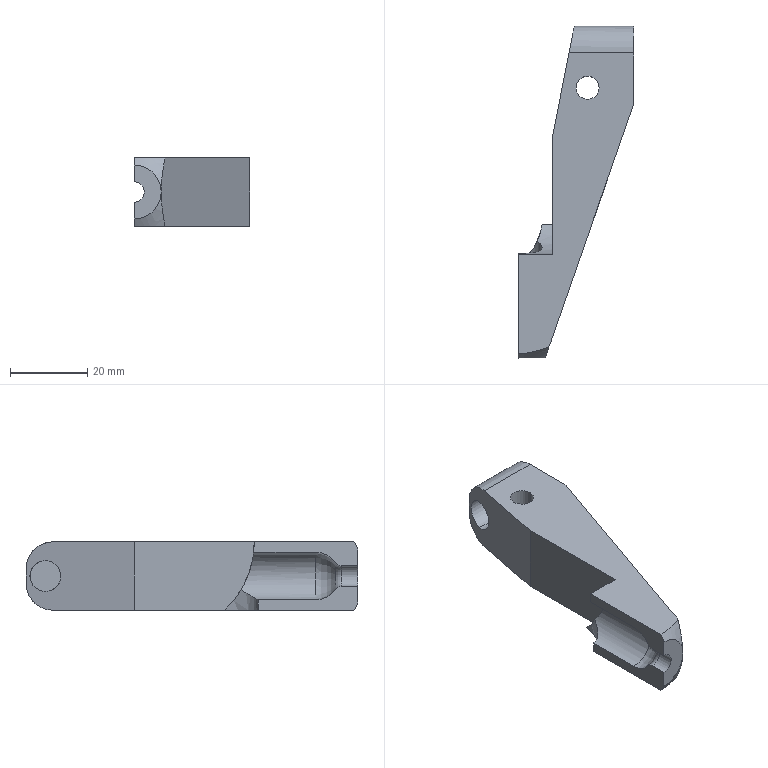Part | SolidWorks | features ICE 6, Extrusion 1, Fillet 1, RevCut 1 | 1 solid | 25 faces | box 30 x 86 x 17.7 mm | volume 18954 mm3 | plane 11 | cylinder 8 | spline 2 | torus 2 | cone 2 | commonest cylinder face diameters 6 x2 8 x2 14 x2 5.3 x1 12.388 x1
STEP:
#1=CARTESIAN_POINT('',(54.,-5.,4.85));
#2=VERTEX_POINT('',#1);
#3=CARTESIAN_POINT('',(54.,-5.,12.85));
#4=VERTEX_POINT('',#3);
#5=CARTESIAN_POINT('',(54.,-5.,8.85));
#6=DIRECTION('',(-1.,0.,0.));
#7=DIRECTION('',(0.,0.,1.));
#8=AXIS2_PLACEMENT_3D('',#5,#6,#7);
#9=CIRCLE('',#8,4.);
#10=EDGE_CURVE('',#2,#4,#9,.T.);
#11=ORIENTED_EDGE('',*,*,#10,.F.);
#12=CARTESIAN_POINT('',(43.6,-5.,4.85));
#13=VERTEX_POINT('',#12);
#14=CARTESIAN_POINT('',(54.,-5.,4.85));
#15=DIRECTION('',(-1.,0.,0.));
#16=VECTOR('',#15,1000.);
#17=LINE('',#14,#16);
#18=EDGE_CURVE('',#2,#13,#17,.T.);
#19=ORIENTED_EDGE('',*,*,#18,.T.);
#20=CARTESIAN_POINT('',(43.6,-5.,12.85));
#21=VERTEX_POINT('',#20);
#22=CARTESIAN_POINT('',(43.6,-5.,12.85));
#23=CARTESIAN_POINT('',(42.,-13.,12.85));
#24=CARTESIAN_POINT('',(42.,-13.,4.85));
#25=CARTESIAN_POINT('',(43.6,-5.,4.85));
#26=(BOUNDED_CURVE()B_SPLINE_CURVE(3,(#22,#23,#24,#25),.UNSPECIFIED.,.F.,.F.)B_SPLINE_CURVE_WITH_KNOTS((4,4),(4.712,7.854),.UNSPECIFIED.)CURVE()GEOMETRIC_REPRESENTATION_ITEM()RATIONAL_B_SPLINE_CURVE((1.,0.3333,0.3333,1.))REPRESENTATION_ITEM(''));
#27=EDGE_CURVE('',#21,#13,#26,.T.);
#28=ORIENTED_EDGE('',*,*,#27,.F.);
#29=CARTESIAN_POINT('',(54.,-5.,12.85));
#30=DIRECTION('',(-1.,0.,0.));
#31=VECTOR('',#30,1000.);
#32=LINE('',#29,#31);
#33=EDGE_CURVE('',#4,#21,#32,.T.);
#34=ORIENTED_EDGE('',*,*,#33,.F.);
#35=EDGE_LOOP('',(#11,#19,#28,#34));
#36=FACE_OUTER_BOUND('',#35,.T.);
#37=CARTESIAN_POINT('',(54.,-5.,8.85));
#38=DIRECTION('',(-1.,0.,0.));
#39=DIRECTION('',(0.,0.,1.));
#40=AXIS2_PLACEMENT_3D('',#37,#38,#39);
#41=CYLINDRICAL_SURFACE('',#40,4.);
#42=ADVANCED_FACE('',(#36),#41,.F.);
#43=CARTESIAN_POINT('',(45.,-16.,17.7));
#44=VERTEX_POINT('',#43);
#45=CARTESIAN_POINT('',(51.,-16.,17.7));
#46=VERTEX_POINT('',#45);
#47=CARTESIAN_POINT('',(48.,-16.,17.7));
#48=DIRECTION('',(0.,0.,1.));
#49=DIRECTION('',(1.,0.,0.));
#50=AXIS2_PLACEMENT_3D('',#47,#48,#49);
#51=CIRCLE('',#50,3.);
#52=EDGE_CURVE('',#44,#46,#51,.T.);
#53=ORIENTED_EDGE('',*,*,#52,.T.);
#54=CARTESIAN_POINT('',(51.,-16.,0.));
#55=VERTEX_POINT('',#54);
#56=CARTESIAN_POINT('',(51.,-16.,17.7));
#57=DIRECTION('',(0.,0.,-1.));
#58=VECTOR('',#57,1000.);
#59=LINE('',#56,#58);
#60=EDGE_CURVE('',#46,#55,#59,.T.);
#61=ORIENTED_EDGE('',*,*,#60,.T.);
#62=CARTESIAN_POINT('',(45.,-16.,0.));
#63=VERTEX_POINT('',#62);
#64=CARTESIAN_POINT('',(48.,-16.,0.));
#65=DIRECTION('',(0.,0.,1.));
#66=DIRECTION('',(1.,0.,0.));
#67=AXIS2_PLACEMENT_3D('',#64,#65,#66);
#68=CIRCLE('',#67,3.);
#69=EDGE_CURVE('',#63,#55,#68,.T.);
#70=ORIENTED_EDGE('',*,*,#69,.F.);
#71=CARTESIAN_POINT('',(45.,-16.,17.7));
#72=DIRECTION('',(0.,0.,-1.));
#73=VECTOR('',#72,1000.);
#74=LINE('',#71,#73);
#75=EDGE_CURVE('',#44,#63,#74,.T.);
#76=ORIENTED_EDGE('',*,*,#75,.F.);
#77=EDGE_LOOP('',(#53,#61,#70,#76));
#78=FACE_OUTER_BOUND('',#77,.T.);
#79=CARTESIAN_POINT('',(48.,-16.,17.7));
#80=DIRECTION('',(0.,0.,-1.));
#81=DIRECTION('',(-1.,0.,0.));
#82=AXIS2_PLACEMENT_3D('',#79,#80,#81);
#83=CYLINDRICAL_SURFACE('',#82,3.);
#84=ADVANCED_FACE('',(#78),#83,.F.);
#85=CARTESIAN_POINT('',(30.,-84.932,17.7));
#86=VERTEX_POINT('',#85);
#87=CARTESIAN_POINT('',(30.,-59.152,17.7));
#88=VERTEX_POINT('',#87);
#89=CARTESIAN_POINT('',(30.,-86.,17.7));
#90=DIRECTION('',(0.,1.,0.));
#91=VECTOR('',#90,1000.);
#92=LINE('',#89,#91);
#93=EDGE_CURVE('',#86,#88,#92,.T.);
#94=ORIENTED_EDGE('',*,*,#93,.F.);
#95=CARTESIAN_POINT('',(37.993,-83.156,17.7));
#96=VERTEX_POINT('',#95);
#97=CARTESIAN_POINT('',(30.,-84.932,17.7));
#98=CARTESIAN_POINT('',(30.683,-84.932,17.7));
#99=CARTESIAN_POINT('',(31.369,-84.886,17.7));
#100=CARTESIAN_POINT('',(32.745,-84.706,17.7));
#101=CARTESIAN_POINT('',(33.421,-84.575,17.7));
#102=CARTESIAN_POINT('',(35.419,-84.091,17.7));
#103=CARTESIAN_POINT('',(36.715,-83.651,17.7));
#104=CARTESIAN_POINT('',(37.993,-83.156,17.7));
#105=B_SPLINE_CURVE_WITH_KNOTS('',3,(#97,#98,#99,#100,#101,#102,#103,#104),.UNSPECIFIED.,.F.,.F.,(4,2,2,4),(0.1214,0.1235,0.1255,0.1297),.UNSPECIFIED.);
#106=EDGE_CURVE('',#86,#96,#105,.T.);
#107=ORIENTED_EDGE('',*,*,#106,.T.);
#108=CARTESIAN_POINT('',(38.331,-82.189,17.7));
#109=VERTEX_POINT('',#108);
#110=CARTESIAN_POINT('',(37.993,-83.156,17.7));
#111=CARTESIAN_POINT('',(38.103,-82.841,17.7));
#112=CARTESIAN_POINT('',(38.216,-82.517,17.7));
#113=CARTESIAN_POINT('',(38.331,-82.189,17.7));
#114=B_SPLINE_CURVE_WITH_KNOTS('',3,(#110,#111,#112,#113),.UNSPECIFIED.,.F.,.F.,(4,4),(0.3587,0.5),.UNSPECIFIED.);
#115=EDGE_CURVE('',#96,#109,#114,.T.);
#116=ORIENTED_EDGE('',*,*,#115,.T.);
#117=CARTESIAN_POINT('',(38.951,-80.412,17.7));
#118=VERTEX_POINT('',#117);
#119=CARTESIAN_POINT('',(38.331,-82.189,17.7));
#120=CARTESIAN_POINT('',(38.533,-81.609,17.7));
#121=CARTESIAN_POINT('',(38.741,-81.014,17.7));
#122=CARTESIAN_POINT('',(38.951,-80.412,17.7));
#123=B_SPLINE_CURVE_WITH_KNOTS('',3,(#119,#120,#121,#122),.UNSPECIFIED.,.F.,.F.,(4,4),(0.,0.25),.UNSPECIFIED.);
#124=EDGE_CURVE('',#109,#118,#123,.T.);
#125=ORIENTED_EDGE('',*,*,#124,.T.);
#126=CARTESIAN_POINT('',(60.,-20.136,17.7));
#127=VERTEX_POINT('',#126);
#128=CARTESIAN_POINT('',(60.,-20.136,17.7));
#129=DIRECTION('',(0.3297,0.9441,0.));
#130=VECTOR('',#129,1000.);
#131=LINE('',#128,#130);
#132=EDGE_CURVE('',#118,#127,#131,.T.);
#133=ORIENTED_EDGE('',*,*,#132,.T.);
#134=CARTESIAN_POINT('',(60.,-7.,17.7));
#135=VERTEX_POINT('',#134);
#136=CARTESIAN_POINT('',(60.,-20.136,17.7));
#137=DIRECTION('',(0.,1.,0.));
#138=VECTOR('',#137,1000.);
#139=LINE('',#136,#138);
#140=EDGE_CURVE('',#127,#135,#139,.T.);
#141=ORIENTED_EDGE('',*,*,#140,.T.);
#142=CARTESIAN_POINT('',(43.2,-7.,17.7));
#143=VERTEX_POINT('',#142);
#144=CARTESIAN_POINT('',(44.6,-7.,17.7));
#145=DIRECTION('',(-1.,0.,0.));
#146=VECTOR('',#145,1000.);
#147=LINE('',#144,#146);
#148=EDGE_CURVE('',#135,#143,#147,.T.);
#149=ORIENTED_EDGE('',*,*,#148,.T.);
#150=CARTESIAN_POINT('',(39.,-28.,17.7));
#151=VERTEX_POINT('',#150);
#152=CARTESIAN_POINT('',(44.6,0.,17.7));
#153=DIRECTION('',(-0.1961,-0.9806,0.));
#154=VECTOR('',#153,1000.);
#155=LINE('',#152,#154);
#156=EDGE_CURVE('',#143,#151,#155,.T.);
#157=ORIENTED_EDGE('',*,*,#156,.T.);
#158=CARTESIAN_POINT('',(39.,-59.152,17.7));
#159=VERTEX_POINT('',#158);
#160=CARTESIAN_POINT('',(39.,-28.,17.7));
#161=DIRECTION('',(0.,-1.,0.));
#162=VECTOR('',#161,1000.);
#163=LINE('',#160,#162);
#164=EDGE_CURVE('',#151,#159,#163,.T.);
#165=ORIENTED_EDGE('',*,*,#164,.T.);
#166=CARTESIAN_POINT('',(58.282,-59.152,17.7));
#167=DIRECTION('',(-1.,0.,0.));
#168=VECTOR('',#167,1000.);
#169=LINE('',#166,#168);
#170=EDGE_CURVE('',#159,#88,#169,.T.);
#171=ORIENTED_EDGE('',*,*,#170,.T.);
#172=EDGE_LOOP('',(#94,#107,#116,#125,#133,#141,#149,#157,#165,#171));
#173=FACE_OUTER_BOUND('',#172,.T.);
#174=ORIENTED_EDGE('',*,*,#52,.F.);
#175=CARTESIAN_POINT('',(48.,-16.,17.7));
#176=DIRECTION('',(0.,0.,1.));
#177=DIRECTION('',(1.,0.,0.));
#178=AXIS2_PLACEMENT_3D('',#175,#176,#177);
#179=CIRCLE('',#178,3.);
#180=EDGE_CURVE('',#46,#44,#179,.T.);
#181=ORIENTED_EDGE('',*,*,#180,.F.);
#182=EDGE_LOOP('',(#174,#181));
#183=FACE_BOUND('',#182,.T.);
#184=CARTESIAN_POINT('',(25.162,-51.504,17.7));
#185=DIRECTION('',(0.,0.,1.));
#186=DIRECTION('',(1.,0.,0.));
#187=AXIS2_PLACEMENT_3D('',#184,#185,#186);
#188=PLANE('',#187);
#189=ADVANCED_FACE('',(#173,#183),#188,.T.);
#190=ORIENTED_EDGE('',*,*,#69,.T.);
#191=CARTESIAN_POINT('',(48.,-16.,0.));
#192=DIRECTION('',(0.,0.,1.));
#193=DIRECTION('',(1.,0.,0.));
#194=AXIS2_PLACEMENT_3D('',#191,#192,#193);
#195=CIRCLE('',#194,3.);
#196=EDGE_CURVE('',#55,#63,#195,.T.);
#197=ORIENTED_EDGE('',*,*,#196,.T.);
#198=EDGE_LOOP('',(#190,#197));
#199=FACE_BOUND('',#198,.T.);
#200=CARTESIAN_POINT('',(30.,-84.932,0.));
#201=VERTEX_POINT('',#200);
#202=CARTESIAN_POINT('',(37.993,-83.156,-0.000000005));
#203=VERTEX_POINT('',#202);
#204=CARTESIAN_POINT('',(30.,-84.932,0.));
#205=CARTESIAN_POINT('',(30.683,-84.932,0.));
#206=CARTESIAN_POINT('',(31.369,-84.886,0.));
#207=CARTESIAN_POINT('',(32.745,-84.706,0.));
#208=CARTESIAN_POINT('',(33.421,-84.575,0.));
#209=CARTESIAN_POINT('',(35.419,-84.091,0.));
#210=CARTESIAN_POINT('',(36.715,-83.651,0.));
#211=CARTESIAN_POINT('',(37.993,-83.156,-0.000000005));
#212=B_SPLINE_CURVE_WITH_KNOTS('',3,(#204,#205,#206,#207,#208,#209,#210,#211),.UNSPECIFIED.,.F.,.F.,(4,2,2,4),(0.1214,0.1235,0.1255,0.1297),.UNSPECIFIED.);
#213=EDGE_CURVE('',#201,#203,#212,.T.);
#214=ORIENTED_EDGE('',*,*,#213,.F.);
#215=CARTESIAN_POINT('',(30.,-60.226,0.));
#216=VERTEX_POINT('',#215);
#217=CARTESIAN_POINT('',(30.,-51.504,0.));
#218=DIRECTION('',(0.,1.,0.));
#219=VECTOR('',#218,1000.);
#220=LINE('',#217,#219);
#221=EDGE_CURVE('',#201,#216,#220,.T.);
#222=ORIENTED_EDGE('',*,*,#221,.T.);
#223=CARTESIAN_POINT('',(36.216,-51.504,0.));
#224=VERTEX_POINT('',#223);
#225=CARTESIAN_POINT('',(36.216,-51.504,0.));
#226=CARTESIAN_POINT('',(35.359,-56.878,0.));
#227=CARTESIAN_POINT('',(32.973,-60.226,0.));
#228=CARTESIAN_POINT('',(30.,-60.226,0.));
#229=(BOUNDED_CURVE()B_SPLINE_CURVE(3,(#225,#226,#227,#228),.UNSPECIFIED.,.F.,.F.)B_SPLINE_CURVE_WITH_KNOTS((4,4),(1.863,3.142),.UNSPECIFIED.)CURVE()GEOMETRIC_REPRESENTATION_ITEM()RATIONAL_B_SPLINE_CURVE((1.,0.8684,0.8684,1.))REPRESENTATION_ITEM(''));
#230=EDGE_CURVE('',#224,#216,#229,.T.);
#231=ORIENTED_EDGE('',*,*,#230,.F.);
#232=CARTESIAN_POINT('',(39.,-51.504,0.));
#233=VERTEX_POINT('',#232);
#234=CARTESIAN_POINT('',(39.,-51.504,0.));
#235=DIRECTION('',(-1.,0.,0.));
#236=VECTOR('',#235,1000.);
#237=LINE('',#234,#236);
#238=EDGE_CURVE('',#233,#224,#237,.T.);
#239=ORIENTED_EDGE('',*,*,#238,.F.);
#240=CARTESIAN_POINT('',(39.,-28.,0.));
#241=VERTEX_POINT('',#240);
#242=CARTESIAN_POINT('',(39.,-28.,0.));
#243=DIRECTION('',(0.,-1.,0.));
#244=VECTOR('',#243,1000.);
#245=LINE('',#242,#244);
#246=EDGE_CURVE('',#241,#233,#245,.T.);
#247=ORIENTED_EDGE('',*,*,#246,.F.);
#248=CARTESIAN_POINT('',(43.2,-7.,0.));
#249=VERTEX_POINT('',#248);
#250=CARTESIAN_POINT('',(44.6,0.,0.));
#251=DIRECTION('',(-0.1961,-0.9806,0.));
#252=VECTOR('',#251,1000.);
#253=LINE('',#250,#252);
#254=EDGE_CURVE('',#249,#241,#253,.T.);
#255=ORIENTED_EDGE('',*,*,#254,.F.);
#256=CARTESIAN_POINT('',(60.,-7.,0.));
#257=VERTEX_POINT('',#256);
#258=CARTESIAN_POINT('',(25.162,-7.,0.));
#259=DIRECTION('',(1.,0.,0.));
#260=VECTOR('',#259,1000.);
#261=LINE('',#258,#260);
#262=EDGE_CURVE('',#249,#257,#261,.T.);
#263=ORIENTED_EDGE('',*,*,#262,.T.);
#264=CARTESIAN_POINT('',(60.,-20.136,0.));
#265=VERTEX_POINT('',#264);
#266=CARTESIAN_POINT('',(60.,-20.136,0.));
#267=DIRECTION('',(0.,1.,0.));
#268=VECTOR('',#267,1000.);
#269=LINE('',#266,#268);
#270=EDGE_CURVE('',#265,#257,#269,.T.);
#271=ORIENTED_EDGE('',*,*,#270,.F.);
#272=CARTESIAN_POINT('',(38.951,-80.412,0.));
#273=VERTEX_POINT('',#272);
#274=CARTESIAN_POINT('',(60.,-20.136,0.));
#275=DIRECTION('',(0.3297,0.9441,0.));
#276=VECTOR('',#275,1000.);
#277=LINE('',#274,#276);
#278=EDGE_CURVE('',#273,#265,#277,.T.);
#279=ORIENTED_EDGE('',*,*,#278,.F.);
#280=CARTESIAN_POINT('',(38.331,-82.189,0.));
#281=VERTEX_POINT('',#280);
#282=CARTESIAN_POINT('',(38.331,-82.189,0.));
#283=CARTESIAN_POINT('',(38.533,-81.609,0.));
#284=CARTESIAN_POINT('',(38.741,-81.014,0.));
#285=CARTESIAN_POINT('',(38.951,-80.412,0.));
#286=B_SPLINE_CURVE_WITH_KNOTS('',3,(#282,#283,#284,#285),.UNSPECIFIED.,.F.,.F.,(4,4),(0.,0.25),.UNSPECIFIED.);
#287=EDGE_CURVE('',#281,#273,#286,.T.);
#288=ORIENTED_EDGE('',*,*,#287,.F.);
#289=CARTESIAN_POINT('',(37.993,-83.156,-0.000000005));
#290=CARTESIAN_POINT('',(38.103,-82.841,0.));
#291=CARTESIAN_POINT('',(38.216,-82.517,0.));
#292=CARTESIAN_POINT('',(38.331,-82.189,0.));
#293=B_SPLINE_CURVE_WITH_KNOTS('',3,(#289,#290,#291,#292),.UNSPECIFIED.,.F.,.F.,(4,4),(0.3587,0.5),.UNSPECIFIED.);
#294=EDGE_CURVE('',#203,#281,#293,.T.);
#295=ORIENTED_EDGE('',*,*,#294,.F.);
#296=EDGE_LOOP('',(#214,#222,#231,#239,#247,#255,#263,#271,#279,#288,#295));
#297=FACE_OUTER_BOUND('',#296,.T.);
#298=CARTESIAN_POINT('',(25.162,-51.504,0.));
#299=DIRECTION('',(0.,0.,1.));
#300=DIRECTION('',(1.,0.,0.));
#301=AXIS2_PLACEMENT_3D('',#298,#299,#300);
#302=PLANE('',#301);
#303=ADVANCED_FACE('',(#199,#297),#302,.F.);
#304=CARTESIAN_POINT('',(37.,-86.,8.85));
#305=VERTEX_POINT('',#304);
#306=CARTESIAN_POINT('',(30.,-86.,15.85));
#307=VERTEX_POINT('',#306);
#308=CARTESIAN_POINT('',(30.,-86.,8.85));
#309=DIRECTION('',(0.,-1.,0.));
#310=DIRECTION('',(0.,0.,-1.));
#311=AXIS2_PLACEMENT_3D('',#308,#309,#310);
#312=CIRCLE('',#311,7.);
#313=EDGE_CURVE('',#305,#307,#312,.T.);
#314=ORIENTED_EDGE('',*,*,#313,.T.);
#315=CARTESIAN_POINT('',(30.,-86.,11.5));
#316=VERTEX_POINT('',#315);
#317=CARTESIAN_POINT('',(30.,-86.,-26.3));
#318=DIRECTION('',(0.,0.,1.));
#319=VECTOR('',#318,1000.);
#320=LINE('',#317,#319);
#321=EDGE_CURVE('',#316,#307,#320,.T.);
#322=ORIENTED_EDGE('',*,*,#321,.F.);
#323=CARTESIAN_POINT('',(30.,-86.,6.2));
#324=VERTEX_POINT('',#323);
#325=CARTESIAN_POINT('',(30.,-86.,8.85));
#326=DIRECTION('',(0.,-1.,0.));
#327=DIRECTION('',(0.,0.,-1.));
#328=AXIS2_PLACEMENT_3D('',#325,#326,#327);
#329=CIRCLE('',#328,2.65);
#330=EDGE_CURVE('',#324,#316,#329,.T.);
#331=ORIENTED_EDGE('',*,*,#330,.F.);
#332=CARTESIAN_POINT('',(30.,-86.,1.85));
#333=VERTEX_POINT('',#332);
#334=CARTESIAN_POINT('',(30.,-86.,-26.3));
#335=DIRECTION('',(0.,0.,1.));
#336=VECTOR('',#335,1000.);
#337=LINE('',#334,#336);
#338=EDGE_CURVE('',#333,#324,#337,.T.);
#339=ORIENTED_EDGE('',*,*,#338,.F.);
#340=CARTESIAN_POINT('',(30.,-86.,8.85));
#341=DIRECTION('',(0.,-1.,0.));
#342=DIRECTION('',(0.,0.,-1.));
#343=AXIS2_PLACEMENT_3D('',#340,#341,#342);
#344=CIRCLE('',#343,7.);
#345=EDGE_CURVE('',#333,#305,#344,.T.);
#346=ORIENTED_EDGE('',*,*,#345,.T.);
#347=EDGE_LOOP('',(#314,#322,#331,#339,#346));
#348=FACE_OUTER_BOUND('',#347,.T.);
#349=CARTESIAN_POINT('',(37.,-86.,17.7));
#350=DIRECTION('',(0.,1.,0.));
#351=DIRECTION('',(0.,0.,1.));
#352=AXIS2_PLACEMENT_3D('',#349,#350,#351);
#353=PLANE('',#352);
#354=ADVANCED_FACE('',(#348),#353,.F.);
#355=CARTESIAN_POINT('',(37.993,-83.156,-0.000000005));
#356=CARTESIAN_POINT('',(37.872,-83.502,0.6974));
#357=CARTESIAN_POINT('',(37.755,-83.838,1.399));
#358=CARTESIAN_POINT('',(37.532,-84.477,2.819));
#359=CARTESIAN_POINT('',(37.426,-84.78,3.537));
#360=CARTESIAN_POINT('',(37.237,-85.321,5.003));
#361=CARTESIAN_POINT('',(37.154,-85.56,5.755));
#362=CARTESIAN_POINT('',(37.035,-85.9,7.28));
#363=CARTESIAN_POINT('',(37.,-86.,8.056));
#364=CARTESIAN_POINT('',(37.,-86.,8.85));
#365=B_SPLINE_CURVE_WITH_KNOTS('',3,(#355,#356,#357,#358,#359,#360,#361,#362,#363,#364),.UNSPECIFIED.,.F.,.F.,(4,2,2,2,4),(0.000000225,0.002359,0.004717,0.007076,0.009434),.UNSPECIFIED.);
#366=EDGE_CURVE('',#203,#305,#365,.T.);
#367=ORIENTED_EDGE('',*,*,#366,.F.);
#368=ORIENTED_EDGE('',*,*,#294,.T.);
#369=ORIENTED_EDGE('',*,*,#287,.T.);
#370=ORIENTED_EDGE('',*,*,#278,.T.);
#371=CARTESIAN_POINT('',(60.,-20.136,17.7));
#372=DIRECTION('',(0.,0.,-1.));
#373=VECTOR('',#372,1000.);
#374=LINE('',#371,#373);
#375=EDGE_CURVE('',#127,#265,#374,.T.);
#376=ORIENTED_EDGE('',*,*,#375,.F.);
#377=ORIENTED_EDGE('',*,*,#132,.F.);
#378=ORIENTED_EDGE('',*,*,#124,.F.);
#379=ORIENTED_EDGE('',*,*,#115,.F.);
#380=CARTESIAN_POINT('',(37.,-86.,8.85));
#381=CARTESIAN_POINT('',(37.,-86.,9.644));
#382=CARTESIAN_POINT('',(37.035,-85.9,10.421));
#383=CARTESIAN_POINT('',(37.154,-85.56,11.945));
#384=CARTESIAN_POINT('',(37.237,-85.321,12.697));
#385=CARTESIAN_POINT('',(37.426,-84.78,14.163));
#386=CARTESIAN_POINT('',(37.532,-84.477,14.881));
#387=CARTESIAN_POINT('',(37.755,-83.838,16.301));
#388=CARTESIAN_POINT('',(37.872,-83.502,17.003));
#389=CARTESIAN_POINT('',(37.993,-83.156,17.7));
#390=B_SPLINE_CURVE_WITH_KNOTS('',3,(#380,#381,#382,#383,#384,#385,#386,#387,#388,#389),.UNSPECIFIED.,.F.,.F.,(4,2,2,2,4),(0.009434,0.01179,0.01415,0.01651,0.01886),.UNSPECIFIED.);
#391=EDGE_CURVE('',#305,#96,#390,.T.);
#392=ORIENTED_EDGE('',*,*,#391,.F.);
#393=EDGE_LOOP('',(#367,#368,#369,#370,#376,#377,#378,#379,#392));
#394=FACE_OUTER_BOUND('',#393,.T.);
#395=CARTESIAN_POINT('',(60.,-20.136,17.7));
#396=DIRECTION('',(-0.9441,0.3297,0.));
#397=DIRECTION('',(-0.3297,-0.9441,0.));
#398=AXIS2_PLACEMENT_3D('',#395,#396,#397);
#399=PLANE('',#398);
#400=ADVANCED_FACE('',(#394),#399,.F.);
#401=CARTESIAN_POINT('',(30.,-75.,2.656));
#402=VERTEX_POINT('',#401);
#403=CARTESIAN_POINT('',(30.,-75.,15.044));
#404=VERTEX_POINT('',#403);
#405=CARTESIAN_POINT('',(30.,-75.,8.85));
#406=DIRECTION('',(0.,-1.,0.));
#407=DIRECTION('',(0.,0.,-1.));
#408=AXIS2_PLACEMENT_3D('',#405,#406,#407);
#409=CIRCLE('',#408,6.194);
#410=EDGE_CURVE('',#402,#404,#409,.T.);
#411=ORIENTED_EDGE('',*,*,#410,.T.);
#412=CARTESIAN_POINT('',(30.,-58.989,15.044));
#413=VERTEX_POINT('',#412);
#414=CARTESIAN_POINT('',(30.,-86.,15.044));
#415=DIRECTION('',(0.,1.,0.));
#416=VECTOR('',#415,1000.);
#417=LINE('',#414,#416);
#418=EDGE_CURVE('',#404,#413,#417,.T.);
#419=ORIENTED_EDGE('',*,*,#418,.T.);
#420=CARTESIAN_POINT('',(35.037,-55.701,5.246));
#421=VERTEX_POINT('',#420);
#422=CARTESIAN_POINT('',(30.,-58.989,15.044));
#423=CARTESIAN_POINT('',(30.294,-58.989,15.044));
#424=CARTESIAN_POINT('',(30.592,-58.987,15.023));
#425=CARTESIAN_POINT('',(31.177,-58.977,14.938));
#426=CARTESIAN_POINT('',(31.464,-58.97,14.876));
#427=CARTESIAN_POINT('',(32.027,-58.95,14.711));
#428=CARTESIAN_POINT('',(32.302,-58.937,14.608));
#429=CARTESIAN_POINT('',(32.842,-58.905,14.362));
#430=CARTESIAN_POINT('',(33.101,-58.885,14.22));
#431=CARTESIAN_POINT('',(33.593,-58.838,13.904));
#432=CARTESIAN_POINT('',(33.827,-58.81,13.729));
#433=CARTESIAN_POINT('',(34.271,-58.744,13.346));
#434=CARTESIAN_POINT('',(34.481,-58.706,13.136));
#435=CARTESIAN_POINT('',(34.864,-58.619,12.697));
#436=CARTESIAN_POINT('',(35.038,-58.571,12.466));
#437=CARTESIAN_POINT('',(35.352,-58.46,11.981));
#438=CARTESIAN_POINT('',(35.493,-58.398,11.726));
#439=CARTESIAN_POINT('',(35.858,-58.193,10.943));
#440=CARTESIAN_POINT('',(36.023,-58.033,10.403));
#441=CARTESIAN_POINT('',(36.204,-57.656,9.292));
#442=CARTESIAN_POINT('',(36.216,-57.441,8.73));
#443=CARTESIAN_POINT('',(36.102,-56.982,7.655));
#444=CARTESIAN_POINT('',(35.976,-56.737,7.137));
#445=CARTESIAN_POINT('',(35.594,-56.221,6.137));
#446=CARTESIAN_POINT('',(35.345,-55.96,5.675));
#447=CARTESIAN_POINT('',(35.037,-55.701,5.246));
#448=B_SPLINE_CURVE_WITH_KNOTS('',3,(#422,#423,#424,#425,#426,#427,#428,#429,#430,#431,#432,#433,#434,#435,#436,#437,#438,#439,#440,#441,#442,#443,#444,#445,#446,#447),.UNSPECIFIED.,.F.,.F.,(4,2,2,2,2,2,2,2,2,2,2,2,4),(0.009865,0.01074,0.01162,0.0125,0.01338,0.01426,0.01514,0.01602,0.0169,0.01866,0.02042,0.02218,0.02394),.UNSPECIFIED.);
#449=EDGE_CURVE('',#413,#421,#448,.T.);
#450=ORIENTED_EDGE('',*,*,#449,.T.);
#451=CARTESIAN_POINT('',(30.,-60.226,2.656));
#452=VERTEX_POINT('',#451);
#453=CARTESIAN_POINT('',(30.,-60.226,2.656));
#454=CARTESIAN_POINT('',(30.16,-60.226,2.656));
#455=CARTESIAN_POINT('',(30.319,-60.215,2.662));
#456=CARTESIAN_POINT('',(30.636,-60.171,2.687));
#457=CARTESIAN_POINT('',(30.794,-60.138,2.705));
#458=CARTESIAN_POINT('',(31.101,-60.052,2.752));
#459=CARTESIAN_POINT('',(31.249,-60.,2.781));
#460=CARTESIAN_POINT('',(31.54,-59.88,2.849));
#461=CARTESIAN_POINT('',(31.682,-59.811,2.887));
#462=CARTESIAN_POINT('',(32.09,-59.586,3.012));
#463=CARTESIAN_POINT('',(32.34,-59.413,3.109));
#464=CARTESIAN_POINT('',(32.807,-59.032,3.322));
#465=CARTESIAN_POINT('',(33.025,-58.823,3.44));
#466=CARTESIAN_POINT('',(33.427,-58.388,3.685));
#467=CARTESIAN_POINT('',(33.612,-58.161,3.814));
#468=CARTESIAN_POINT('',(33.958,-57.693,4.081));
#469=CARTESIAN_POINT('',(34.119,-57.45,4.22));
#470=CARTESIAN_POINT('',(34.566,-56.714,4.645));
#471=CARTESIAN_POINT('',(34.818,-56.21,4.939));
#472=CARTESIAN_POINT('',(35.037,-55.701,5.246));
#473=B_SPLINE_CURVE_WITH_KNOTS('',3,(#453,#454,#455,#456,#457,#458,#459,#460,#461,#462,#463,#464,#465,#466,#467,#468,#469,#470,#471,#472),.UNSPECIFIED.,.F.,.F.,(4,2,2,2,2,2,2,2,2,4),(0.005376,0.005854,0.006331,0.006809,0.007286,0.008241,0.009196,0.01015,0.01111,0.01302),.UNSPECIFIED.);
#474=EDGE_CURVE('',#452,#421,#473,.T.);
#475=ORIENTED_EDGE('',*,*,#474,.F.);
#476=CARTESIAN_POINT('',(30.,-86.,2.656));
#477=DIRECTION('',(0.,-1.,0.));
#478=VECTOR('',#477,1000.);
#479=LINE('',#476,#478);
#480=EDGE_CURVE('',#452,#402,#479,.T.);
#481=ORIENTED_EDGE('',*,*,#480,.T.);
#482=EDGE_LOOP('',(#411,#419,#450,#475,#481));
#483=FACE_OUTER_BOUND('',#482,.T.);
#484=CARTESIAN_POINT('',(30.,-86.,8.85));
#485=DIRECTION('',(0.,-1.,0.));
#486=DIRECTION('',(0.,0.,-1.));
#487=AXIS2_PLACEMENT_3D('',#484,#485,#486);
#488=CYLINDRICAL_SURFACE('',#487,6.194);
#489=ADVANCED_FACE('',(#483),#488,.F.);
#490=ORIENTED_EDGE('',*,*,#449,.F.);
#491=CARTESIAN_POINT('',(30.,-58.989,15.044));
#492=CARTESIAN_POINT('',(30.,-59.134,16.346));
#493=CARTESIAN_POINT('',(30.,-59.152,17.7));
#494=B_SPLINE_CURVE_WITH_KNOTS('',2,(#491,#492,#493),.UNSPECIFIED.,.F.,.F.,(3,3),(0.8694,1.),.UNSPECIFIED.);
#495=EDGE_CURVE('',#413,#88,#494,.T.);
#496=ORIENTED_EDGE('',*,*,#495,.T.);
#497=ORIENTED_EDGE('',*,*,#170,.F.);
#498=CARTESIAN_POINT('',(39.,-51.504,0.));
#499=CARTESIAN_POINT('',(39.,-59.009,7.335));
#500=CARTESIAN_POINT('',(39.,-59.152,17.7));
#501=B_SPLINE_CURVE_WITH_KNOTS('',2,(#498,#499,#500),.UNSPECIFIED.,.F.,.F.,(3,3),(0.,1.),.UNSPECIFIED.);
#502=EDGE_CURVE('',#233,#159,#501,.T.);
#503=ORIENTED_EDGE('',*,*,#502,.F.);
#504=ORIENTED_EDGE('',*,*,#238,.T.);
#505=CARTESIAN_POINT('',(35.037,-55.701,5.246));
#506=CARTESIAN_POINT('',(35.285,-55.125,4.293));
#507=CARTESIAN_POINT('',(35.516,-54.482,3.378));
#508=CARTESIAN_POINT('',(35.917,-53.075,1.625));
#509=CARTESIAN_POINT('',(36.087,-52.315,0.7934));
#510=CARTESIAN_POINT('',(36.216,-51.504,0.));
#511=B_SPLINE_CURVE_WITH_KNOTS('',3,(#505,#506,#507,#508,#509,#510),.UNSPECIFIED.,.F.,.F.,(4,2,4),(0.00413,0.007549,0.01097),.UNSPECIFIED.);
#512=EDGE_CURVE('',#421,#224,#511,.T.);
#513=ORIENTED_EDGE('',*,*,#512,.F.);
#514=EDGE_LOOP('',(#490,#496,#497,#503,#504,#513));
#515=FACE_OUTER_BOUND('',#514,.T.);
#516=CARTESIAN_POINT('',(39.,-51.504,0.));
#517=CARTESIAN_POINT('',(30.,-51.504,0.));
#518=CARTESIAN_POINT('',(39.,-59.009,7.335));
#519=CARTESIAN_POINT('',(30.,-59.009,7.335));
#520=CARTESIAN_POINT('',(39.,-59.152,17.7));
#521=CARTESIAN_POINT('',(30.,-59.152,17.7));
#522=B_SPLINE_SURFACE_WITH_KNOTS('',2,1,((#516,#517),(#518,#519),(#520,#521)),.UNSPECIFIED.,.F.,.F.,.F.,(3,3),(2,2),(0.,1.),(0.,1.),.UNSPECIFIED.);
#523=ADVANCED_FACE('',(#515),#522,.F.);
#524=CARTESIAN_POINT('',(60.,0.,10.7));
#525=VERTEX_POINT('',#524);
#526=CARTESIAN_POINT('',(60.,0.,7.));
#527=VERTEX_POINT('',#526);
#528=CARTESIAN_POINT('',(60.,0.,17.7));
#529=DIRECTION('',(0.,0.,-1.));
#530=VECTOR('',#529,1000.);
#531=LINE('',#528,#530);
#532=EDGE_CURVE('',#525,#527,#531,.T.);
#533=ORIENTED_EDGE('',*,*,#532,.F.);
#534=CARTESIAN_POINT('',(60.,-7.,10.7));
#535=DIRECTION('',(1.,0.,0.));
#536=DIRECTION('',(0.,0.,1.));
#537=AXIS2_PLACEMENT_3D('',#534,#535,#536);
#538=CIRCLE('',#537,7.);
#539=EDGE_CURVE('',#525,#135,#538,.T.);
#540=ORIENTED_EDGE('',*,*,#539,.T.);
#541=ORIENTED_EDGE('',*,*,#140,.F.);
#542=ORIENTED_EDGE('',*,*,#375,.T.);
#543=ORIENTED_EDGE('',*,*,#270,.T.);
#544=CARTESIAN_POINT('',(60.,-7.,7.));
#545=DIRECTION('',(1.,0.,0.));
#546=DIRECTION('',(0.,0.,1.));
#547=AXIS2_PLACEMENT_3D('',#544,#545,#546);
#548=CIRCLE('',#547,7.);
#549=EDGE_CURVE('',#257,#527,#548,.T.);
#550=ORIENTED_EDGE('',*,*,#549,.T.);
#551=EDGE_LOOP('',(#533,#540,#541,#542,#543,#550));
#552=FACE_OUTER_BOUND('',#551,.T.);
#553=CARTESIAN_POINT('',(60.,-20.136,17.7));
#554=DIRECTION('',(-1.,0.,0.));
#555=DIRECTION('',(0.,0.,1.));
#556=AXIS2_PLACEMENT_3D('',#553,#554,#555);
#557=PLANE('',#556);
#558=ADVANCED_FACE('',(#552),#557,.F.);
#559=CARTESIAN_POINT('',(44.6,0.,10.7));
#560=VERTEX_POINT('',#559);
#561=CARTESIAN_POINT('',(44.6,0.,7.));
#562=VERTEX_POINT('',#561);
#563=CARTESIAN_POINT('',(44.6,0.,17.7));
#564=DIRECTION('',(0.,0.,-1.));
#565=VECTOR('',#564,1000.);
#566=LINE('',#563,#565);
#567=EDGE_CURVE('',#560,#562,#566,.T.);
#568=ORIENTED_EDGE('',*,*,#567,.F.);
#569=CARTESIAN_POINT('',(60.,0.,10.7));
#570=DIRECTION('',(1.,0.,0.));
#571=VECTOR('',#570,1000.);
#572=LINE('',#569,#571);
#573=EDGE_CURVE('',#560,#525,#572,.T.);
#574=ORIENTED_EDGE('',*,*,#573,.T.);
#575=ORIENTED_EDGE('',*,*,#532,.T.);
#576=CARTESIAN_POINT('',(60.,0.,7.));
#577=DIRECTION('',(-1.,0.,0.));
#578=VECTOR('',#577,1000.);
#579=LINE('',#576,#578);
#580=EDGE_CURVE('',#527,#562,#579,.T.);
#581=ORIENTED_EDGE('',*,*,#580,.T.);
#582=EDGE_LOOP('',(#568,#574,#575,#581));
#583=FACE_OUTER_BOUND('',#582,.T.);
#584=CARTESIAN_POINT('',(60.,0.,17.7));
#585=DIRECTION('',(0.,-1.,0.));
#586=DIRECTION('',(0.,0.,-1.));
#587=AXIS2_PLACEMENT_3D('',#584,#585,#586);
#588=PLANE('',#587);
#589=ADVANCED_FACE('',(#583),#588,.F.);
#590=ORIENTED_EDGE('',*,*,#27,.T.);
#591=CARTESIAN_POINT('',(43.6,-5.,4.85));
#592=CARTESIAN_POINT('',(45.2,3.,4.85));
#593=CARTESIAN_POINT('',(45.2,3.,12.85));
#594=CARTESIAN_POINT('',(43.6,-5.,12.85));
#595=(BOUNDED_CURVE()B_SPLINE_CURVE(3,(#591,#592,#593,#594),.UNSPECIFIED.,.F.,.F.)B_SPLINE_CURVE_WITH_KNOTS((4,4),(1.571,4.712),.UNSPECIFIED.)CURVE()GEOMETRIC_REPRESENTATION_ITEM()RATIONAL_B_SPLINE_CURVE((1.,0.3333,0.3333,1.))REPRESENTATION_ITEM(''));
#596=EDGE_CURVE('',#13,#21,#595,.T.);
#597=ORIENTED_EDGE('',*,*,#596,.T.);
#598=EDGE_LOOP('',(#590,#597));
#599=FACE_BOUND('',#598,.T.);
#600=ORIENTED_EDGE('',*,*,#156,.F.);
#601=CARTESIAN_POINT('',(43.2,-7.,17.7));
#602=CARTESIAN_POINT('',(44.02,-2.899,17.7));
#603=CARTESIAN_POINT('',(44.6,0.,14.801));
#604=CARTESIAN_POINT('',(44.6,0.,10.7));
#605=(BOUNDED_CURVE()B_SPLINE_CURVE(3,(#601,#602,#603,#604),.UNSPECIFIED.,.F.,.F.)B_SPLINE_CURVE_WITH_KNOTS((4,4),(4.712,6.283),.UNSPECIFIED.)CURVE()GEOMETRIC_REPRESENTATION_ITEM()RATIONAL_B_SPLINE_CURVE((1.,0.8047,0.8047,1.))REPRESENTATION_ITEM(''));
#606=EDGE_CURVE('',#143,#560,#605,.T.);
#607=ORIENTED_EDGE('',*,*,#606,.T.);
#608=ORIENTED_EDGE('',*,*,#567,.T.);
#609=CARTESIAN_POINT('',(44.6,0.,7.));
#610=CARTESIAN_POINT('',(44.6,0.,2.899));
#611=CARTESIAN_POINT('',(44.02,-2.899,0.));
#612=CARTESIAN_POINT('',(43.2,-7.,0.));
#613=(BOUNDED_CURVE()B_SPLINE_CURVE(3,(#609,#610,#611,#612),.UNSPECIFIED.,.F.,.F.)B_SPLINE_CURVE_WITH_KNOTS((4,4),(3.142,4.712),.UNSPECIFIED.)CURVE()GEOMETRIC_REPRESENTATION_ITEM()RATIONAL_B_SPLINE_CURVE((1.,0.8047,0.8047,1.))REPRESENTATION_ITEM(''));
#614=EDGE_CURVE('',#562,#249,#613,.T.);
#615=ORIENTED_EDGE('',*,*,#614,.T.);
#616=ORIENTED_EDGE('',*,*,#254,.T.);
#617=CARTESIAN_POINT('',(39.,-28.,17.7));
#618=DIRECTION('',(0.,0.,-1.));
#619=VECTOR('',#618,1000.);
#620=LINE('',#617,#619);
#621=EDGE_CURVE('',#151,#241,#620,.T.);
#622=ORIENTED_EDGE('',*,*,#621,.F.);
#623=EDGE_LOOP('',(#600,#607,#608,#615,#616,#622));
#624=FACE_OUTER_BOUND('',#623,.T.);
#625=CARTESIAN_POINT('',(44.6,0.,17.7));
#626=DIRECTION('',(0.9806,-0.1961,0.));
#627=DIRECTION('',(0.1961,0.9806,0.));
#628=AXIS2_PLACEMENT_3D('',#625,#626,#627);
#629=PLANE('',#628);
#630=ADVANCED_FACE('',(#599,#624),#629,.F.);
#631=ORIENTED_EDGE('',*,*,#246,.T.);
#632=ORIENTED_EDGE('',*,*,#502,.T.);
#633=ORIENTED_EDGE('',*,*,#164,.F.);
#634=ORIENTED_EDGE('',*,*,#621,.T.);
#635=EDGE_LOOP('',(#631,#632,#633,#634));
#636=FACE_OUTER_BOUND('',#635,.T.);
#637=CARTESIAN_POINT('',(39.,-28.,17.7));
#638=DIRECTION('',(1.,0.,0.));
#639=DIRECTION('',(0.,0.,-1.));
#640=AXIS2_PLACEMENT_3D('',#637,#638,#639);
#641=PLANE('',#640);
#642=ADVANCED_FACE('',(#636),#641,.F.);
#643=ORIENTED_EDGE('',*,*,#60,.F.);
#644=ORIENTED_EDGE('',*,*,#180,.T.);
#645=ORIENTED_EDGE('',*,*,#75,.T.);
#646=ORIENTED_EDGE('',*,*,#196,.F.);
#647=EDGE_LOOP('',(#643,#644,#645,#646));
#648=FACE_OUTER_BOUND('',#647,.T.);
#649=CARTESIAN_POINT('',(48.,-16.,17.7));
#650=DIRECTION('',(0.,0.,-1.));
#651=DIRECTION('',(-1.,0.,0.));
#652=AXIS2_PLACEMENT_3D('',#649,#650,#651);
#653=CYLINDRICAL_SURFACE('',#652,3.);
#654=ADVANCED_FACE('',(#648),#653,.F.);
#655=CARTESIAN_POINT('',(30.,-81.75,6.2));
#656=VERTEX_POINT('',#655);
#657=CARTESIAN_POINT('',(30.,-81.75,11.5));
#658=VERTEX_POINT('',#657);
#659=CARTESIAN_POINT('',(30.,-81.75,8.85));
#660=DIRECTION('',(0.,-1.,0.));
#661=DIRECTION('',(0.,0.,-1.));
#662=AXIS2_PLACEMENT_3D('',#659,#660,#661);
#663=CIRCLE('',#662,2.65);
#664=EDGE_CURVE('',#656,#658,#663,.T.);
#665=ORIENTED_EDGE('',*,*,#664,.T.);
#666=CARTESIAN_POINT('',(30.,-80.104,12.364));
#667=VERTEX_POINT('',#666);
#668=CARTESIAN_POINT('',(30.,-81.75,13.5));
#669=DIRECTION('',(1.,0.,0.));
#670=DIRECTION('',(0.,0.,-1.));
#671=AXIS2_PLACEMENT_3D('',#668,#669,#670);
#672=CIRCLE('',#671,2.);
#673=EDGE_CURVE('',#658,#667,#672,.T.);
#674=ORIENTED_EDGE('',*,*,#673,.T.);
#675=CARTESIAN_POINT('',(30.,-80.104,5.336));
#676=VERTEX_POINT('',#675);
#677=CARTESIAN_POINT('',(30.,-80.104,8.85));
#678=DIRECTION('',(0.,-1.,0.));
#679=DIRECTION('',(0.,0.,-1.));
#680=AXIS2_PLACEMENT_3D('',#677,#678,#679);
#681=CIRCLE('',#680,3.514);
#682=EDGE_CURVE('',#676,#667,#681,.T.);
#683=ORIENTED_EDGE('',*,*,#682,.F.);
#684=CARTESIAN_POINT('',(30.,-81.75,4.2));
#685=DIRECTION('',(1.,0.,0.));
#686=DIRECTION('',(0.,0.,-1.));
#687=AXIS2_PLACEMENT_3D('',#684,#685,#686);
#688=CIRCLE('',#687,2.);
#689=EDGE_CURVE('',#676,#656,#688,.T.);
#690=ORIENTED_EDGE('',*,*,#689,.T.);
#691=EDGE_LOOP('',(#665,#674,#683,#690));
#692=FACE_OUTER_BOUND('',#691,.T.);
#693=CARTESIAN_POINT('',(30.,-81.75,8.85));
#694=DIRECTION('',(0.,-1.,0.));
#695=DIRECTION('',(0.,0.,-1.));
#696=AXIS2_PLACEMENT_3D('',#693,#694,#695);
#697=TOROIDAL_SURFACE('',#696,4.65,2.);
#698=ADVANCED_FACE('',(#692),#697,.T.);
#699=ORIENTED_EDGE('',*,*,#682,.T.);
#700=CARTESIAN_POINT('',(30.,-75.,8.844));
#701=DIRECTION('',(-1.,0.,0.));
#702=DIRECTION('',(0.,0.,-1.));
#703=AXIS2_PLACEMENT_3D('',#700,#701,#702);
#704=CIRCLE('',#703,6.2);
#705=EDGE_CURVE('',#667,#404,#704,.T.);
#706=ORIENTED_EDGE('',*,*,#705,.T.);
#707=ORIENTED_EDGE('',*,*,#410,.F.);
#708=CARTESIAN_POINT('',(30.,-75.,8.856));
#709=DIRECTION('',(-1.,0.,0.));
#710=DIRECTION('',(0.,0.,-1.));
#711=AXIS2_PLACEMENT_3D('',#708,#709,#710);
#712=CIRCLE('',#711,6.2);
#713=EDGE_CURVE('',#402,#676,#712,.T.);
#714=ORIENTED_EDGE('',*,*,#713,.T.);
#715=EDGE_LOOP('',(#699,#706,#707,#714));
#716=FACE_OUTER_BOUND('',#715,.T.);
#717=CARTESIAN_POINT('',(30.,-75.,8.85));
#718=DIRECTION('',(0.,-1.,0.));
#719=DIRECTION('',(0.,0.,-1.));
#720=AXIS2_PLACEMENT_3D('',#717,#718,#719);
#721=TOROIDAL_SURFACE('',#720,-0.00591,6.2);
#722=ADVANCED_FACE('',(#716),#721,.F.);
#723=ORIENTED_EDGE('',*,*,#330,.T.);
#724=CARTESIAN_POINT('',(30.,-86.,11.5));
#725=DIRECTION('',(0.,1.,0.));
#726=VECTOR('',#725,1000.);
#727=LINE('',#724,#726);
#728=EDGE_CURVE('',#316,#658,#727,.T.);
#729=ORIENTED_EDGE('',*,*,#728,.T.);
#730=ORIENTED_EDGE('',*,*,#664,.F.);
#731=CARTESIAN_POINT('',(30.,-86.,6.2));
#732=DIRECTION('',(0.,-1.,0.));
#733=VECTOR('',#732,1000.);
#734=LINE('',#731,#733);
#735=EDGE_CURVE('',#656,#324,#734,.T.);
#736=ORIENTED_EDGE('',*,*,#735,.T.);
#737=EDGE_LOOP('',(#723,#729,#730,#736));
#738=FACE_OUTER_BOUND('',#737,.T.);
#739=CARTESIAN_POINT('',(30.,-86.,8.85));
#740=DIRECTION('',(0.,-1.,0.));
#741=DIRECTION('',(0.,0.,-1.));
#742=AXIS2_PLACEMENT_3D('',#739,#740,#741);
#743=CYLINDRICAL_SURFACE('',#742,2.65);
#744=ADVANCED_FACE('',(#738),#743,.F.);
#745=CARTESIAN_POINT('',(30.,-60.226,2.639));
#746=DIRECTION('',(0.,0.,-1.));
#747=VECTOR('',#746,1000.);
#748=LINE('',#745,#747);
#749=EDGE_CURVE('',#452,#216,#748,.T.);
#750=ORIENTED_EDGE('',*,*,#749,.F.);
#751=ORIENTED_EDGE('',*,*,#474,.T.);
#752=ORIENTED_EDGE('',*,*,#512,.T.);
#753=ORIENTED_EDGE('',*,*,#230,.T.);
#754=EDGE_LOOP('',(#750,#751,#752,#753));
#755=FACE_OUTER_BOUND('',#754,.T.);
#756=CARTESIAN_POINT('',(36.23,-51.413,0.));
#757=CARTESIAN_POINT('',(36.23,-51.413,5.277));
#758=CARTESIAN_POINT('',(35.389,-56.838,0.));
#759=CARTESIAN_POINT('',(35.389,-56.838,5.277));
#760=CARTESIAN_POINT('',(32.993,-60.226,0.));
#761=CARTESIAN_POINT('',(32.993,-60.226,5.277));
#762=CARTESIAN_POINT('',(30.,-60.226,0.));
#763=CARTESIAN_POINT('',(30.,-60.226,5.277));
#764=(BOUNDED_SURFACE()B_SPLINE_SURFACE(3,1,((#756,#757),(#758,#759),(#760,#761),(#762,#763)),.UNSPECIFIED.,.F.,.F.,.F.)B_SPLINE_SURFACE_WITH_KNOTS((4,4),(2,2),(0.,1.),(0.,1.),.UNSPECIFIED.)GEOMETRIC_REPRESENTATION_ITEM()RATIONAL_B_SPLINE_SURFACE(((1.,1.),(0.8669,0.8669),(0.8669,0.8669),(1.,1.)))REPRESENTATION_ITEM('')SURFACE());
#765=ADVANCED_FACE('',(#755),#764,.T.);
#766=CARTESIAN_POINT('',(54.,-5.,8.85));
#767=DIRECTION('',(-1.,0.,0.));
#768=DIRECTION('',(0.,0.,1.));
#769=AXIS2_PLACEMENT_3D('',#766,#767,#768);
#770=CIRCLE('',#769,4.);
#771=EDGE_CURVE('',#4,#2,#770,.T.);
#772=ORIENTED_EDGE('',*,*,#771,.T.);
#773=ORIENTED_EDGE('',*,*,#10,.T.);
#774=EDGE_LOOP('',(#772,#773));
#775=FACE_OUTER_BOUND('',#774,.T.);
#776=CARTESIAN_POINT('',(54.,-5.,8.85));
#777=DIRECTION('',(-1.,0.,0.));
#778=DIRECTION('',(0.,0.,1.));
#779=AXIS2_PLACEMENT_3D('',#776,#777,#778);
#780=PLANE('',#779);
#781=ADVANCED_FACE('',(#775),#780,.T.);
#782=ORIENTED_EDGE('',*,*,#18,.F.);
#783=ORIENTED_EDGE('',*,*,#771,.F.);
#784=ORIENTED_EDGE('',*,*,#33,.T.);
#785=ORIENTED_EDGE('',*,*,#596,.F.);
#786=EDGE_LOOP('',(#782,#783,#784,#785));
#787=FACE_OUTER_BOUND('',#786,.T.);
#788=CARTESIAN_POINT('',(54.,-5.,8.85));
#789=DIRECTION('',(-1.,0.,0.));
#790=DIRECTION('',(0.,0.,1.));
#791=AXIS2_PLACEMENT_3D('',#788,#789,#790);
#792=CYLINDRICAL_SURFACE('',#791,4.);
#793=ADVANCED_FACE('',(#787),#792,.F.);
#794=ORIENTED_EDGE('',*,*,#539,.F.);
#795=ORIENTED_EDGE('',*,*,#573,.F.);
#796=ORIENTED_EDGE('',*,*,#606,.F.);
#797=ORIENTED_EDGE('',*,*,#148,.F.);
#798=EDGE_LOOP('',(#794,#795,#796,#797));
#799=FACE_OUTER_BOUND('',#798,.T.);
#800=CARTESIAN_POINT('',(25.162,-7.,10.7));
#801=DIRECTION('',(1.,0.,0.));
#802=DIRECTION('',(0.,0.,-1.));
#803=AXIS2_PLACEMENT_3D('',#800,#801,#802);
#804=CYLINDRICAL_SURFACE('',#803,7.);
#805=ADVANCED_FACE('',(#799),#804,.T.);
#806=ORIENTED_EDGE('',*,*,#549,.F.);
#807=ORIENTED_EDGE('',*,*,#262,.F.);
#808=ORIENTED_EDGE('',*,*,#614,.F.);
#809=ORIENTED_EDGE('',*,*,#580,.F.);
#810=EDGE_LOOP('',(#806,#807,#808,#809));
#811=FACE_OUTER_BOUND('',#810,.T.);
#812=CARTESIAN_POINT('',(60.,-7.,7.));
#813=DIRECTION('',(-1.,0.,0.));
#814=DIRECTION('',(0.,0.,1.));
#815=AXIS2_PLACEMENT_3D('',#812,#813,#814);
#816=CYLINDRICAL_SURFACE('',#815,7.);
#817=ADVANCED_FACE('',(#811),#816,.T.);
#818=CARTESIAN_POINT('',(30.,-90.041,8.85));
#819=DIRECTION('',(0.,0.5,0.866));
#820=VECTOR('',#819,1000.);
#821=LINE('',#818,#820);
#822=EDGE_CURVE('',#307,#86,#821,.T.);
#823=ORIENTED_EDGE('',*,*,#822,.F.);
#824=ORIENTED_EDGE('',*,*,#313,.F.);
#825=ORIENTED_EDGE('',*,*,#391,.T.);
#826=ORIENTED_EDGE('',*,*,#106,.F.);
#827=EDGE_LOOP('',(#823,#824,#825,#826));
#828=FACE_OUTER_BOUND('',#827,.T.);
#829=CARTESIAN_POINT('',(30.,-86.,8.85));
#830=DIRECTION('',(0.,1.,0.));
#831=DIRECTION('',(0.,0.,-1.));
#832=AXIS2_PLACEMENT_3D('',#829,#830,#831);
#833=CONICAL_SURFACE('',#832,7.,1.047);
#834=ADVANCED_FACE('',(#828),#833,.T.);
#835=CARTESIAN_POINT('',(30.,-90.041,8.85));
#836=DIRECTION('',(0.,-0.5,0.866));
#837=VECTOR('',#836,1000.);
#838=LINE('',#835,#837);
#839=EDGE_CURVE('',#201,#333,#838,.T.);
#840=ORIENTED_EDGE('',*,*,#839,.F.);
#841=ORIENTED_EDGE('',*,*,#213,.T.);
#842=ORIENTED_EDGE('',*,*,#366,.T.);
#843=ORIENTED_EDGE('',*,*,#345,.F.);
#844=EDGE_LOOP('',(#840,#841,#842,#843));
#845=FACE_OUTER_BOUND('',#844,.T.);
#846=CARTESIAN_POINT('',(30.,-86.,8.85));
#847=DIRECTION('',(0.,1.,0.));
#848=DIRECTION('',(0.,0.,-1.));
#849=AXIS2_PLACEMENT_3D('',#846,#847,#848);
#850=CONICAL_SURFACE('',#849,7.,1.047);
#851=ADVANCED_FACE('',(#845),#850,.T.);
#852=ORIENTED_EDGE('',*,*,#689,.F.);
#853=ORIENTED_EDGE('',*,*,#713,.F.);
#854=ORIENTED_EDGE('',*,*,#480,.F.);
#855=ORIENTED_EDGE('',*,*,#749,.T.);
#856=ORIENTED_EDGE('',*,*,#221,.F.);
#857=ORIENTED_EDGE('',*,*,#839,.T.);
#858=ORIENTED_EDGE('',*,*,#338,.T.);
#859=ORIENTED_EDGE('',*,*,#735,.F.);
#860=EDGE_LOOP('',(#852,#853,#854,#855,#856,#857,#858,#859));
#861=FACE_OUTER_BOUND('',#860,.T.);
#862=CARTESIAN_POINT('',(30.,-86.,-26.3));
#863=DIRECTION('',(1.,0.,0.));
#864=DIRECTION('',(0.,0.,-1.));
#865=AXIS2_PLACEMENT_3D('',#862,#863,#864);
#866=PLANE('',#865);
#867=ADVANCED_FACE('',(#861),#866,.F.);
#868=ORIENTED_EDGE('',*,*,#418,.F.);
#869=ORIENTED_EDGE('',*,*,#705,.F.);
#870=ORIENTED_EDGE('',*,*,#673,.F.);
#871=ORIENTED_EDGE('',*,*,#728,.F.);
#872=ORIENTED_EDGE('',*,*,#321,.T.);
#873=ORIENTED_EDGE('',*,*,#822,.T.);
#874=ORIENTED_EDGE('',*,*,#93,.T.);
#875=ORIENTED_EDGE('',*,*,#495,.F.);
#876=EDGE_LOOP('',(#868,#869,#870,#871,#872,#873,#874,#875));
#877=FACE_OUTER_BOUND('',#876,.T.);
#878=CARTESIAN_POINT('',(30.,-86.,-26.3));
#879=DIRECTION('',(1.,0.,0.));
#880=DIRECTION('',(0.,0.,-1.));
#881=AXIS2_PLACEMENT_3D('',#878,#879,#880);
#882=PLANE('',#881);
#883=ADVANCED_FACE('',(#877),#882,.F.);
#884=CLOSED_SHELL('',(#42,#84,#189,#303,#354,#400,#489,#523,#558,#589,#630,#642,#654,#698,#722,#744,#765,#781,#793,#805,#817,#834,#851,#867,#883));
#885=MANIFOLD_SOLID_BREP('',#884);
#886=CARTESIAN_POINT('',(0.,0.,0.));
#887=DIRECTION('',(0.,0.,1.));
#888=DIRECTION('',(1.,0.,0.));
#889=AXIS2_PLACEMENT_3D('',#886,#887,#888);
#890=(LENGTH_UNIT()NAMED_UNIT(*)SI_UNIT(.MILLI.,.METRE.));
#891=UNCERTAINTY_MEASURE_WITH_UNIT(LENGTH_MEASURE(0.00001),#890,'','');
#892=(NAMED_UNIT(*)PLANE_ANGLE_UNIT()SI_UNIT($,.RADIAN.));
#893=(NAMED_UNIT(*)SI_UNIT($,.STERADIAN.)SOLID_ANGLE_UNIT());
#894=(GEOMETRIC_REPRESENTATION_CONTEXT(3)GLOBAL_UNCERTAINTY_ASSIGNED_CONTEXT((#891))GLOBAL_UNIT_ASSIGNED_CONTEXT((#890,#892,#893))REPRESENTATION_CONTEXT('',''));
#895=ADVANCED_BREP_SHAPE_REPRESENTATION('',(#885,#889),#894);